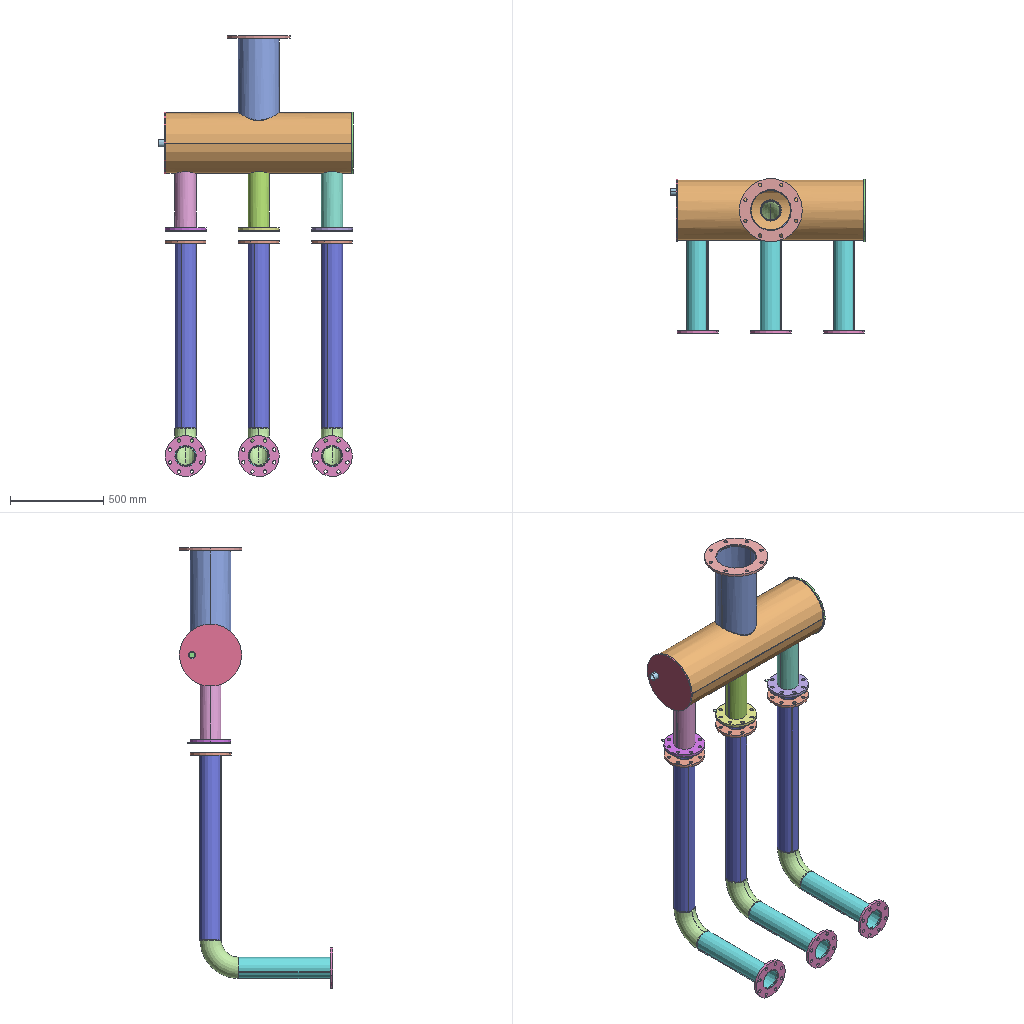Assembly | SolidWorks | 7 different items | 16 placed | box 1046 x 824 x 2365 mm
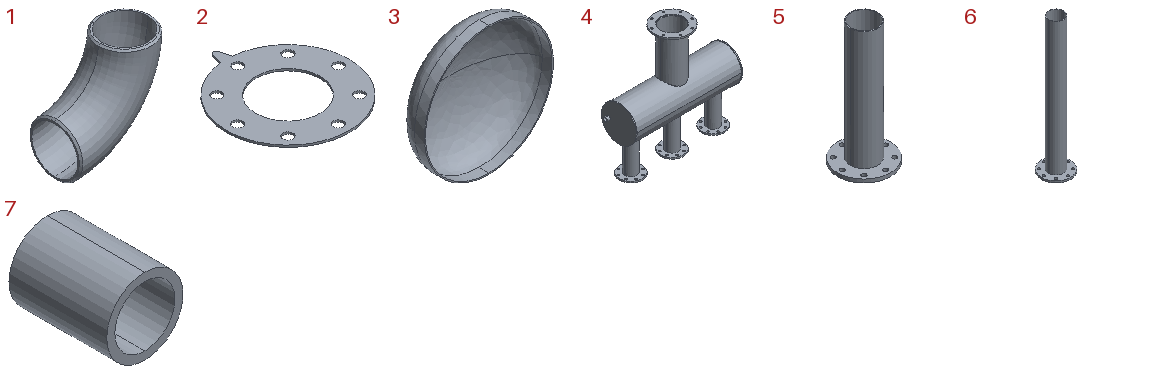Parts list (item | quantity | size | volume | features):
1 | x3 | 209.12 x 114.3 x 209.115 mm | 569487 mm3 | features Chamfer 1, Revolution 1
2 | x3 | 220 x 243.233 x 3.5 mm | 90689 mm3 | features Extrusion 1
3 | x2 | 325 x 106 x 325 mm | 399345 mm3 | features Revolution 2
4 | x1 | 1046 x 340 x 1046 mm | 7874309 mm3 | features ICE 8, 3DProfileFeature 4, Extrusion 1, MoveCopyBody 1, Stock 1, Sweep 1, WeldmentFeature 1
5 | x3 | 220 x 220 x 504 mm | 882758 mm3 | features Extrusion 1, ICE 1
6 | x3 | 220 x 220 x 1004 mm | 1407247 mm3 | features Extrusion 1, ICE 1
7 | x1 | 39 x 50 x 39 mm | 22597 mm3 | features 3DProfileFeature 1, Extrusion 1, HoleWzd 1
Mates (type | each side: item.copy, entity, surface, feature):
Concentric | 4.1 edge | 2.1 edge
Coincident | 4.1 face plane Boss-Extrude5 | 2.1 face plane Boss-Extrude1
Concentric | 4.1 face cylinder Boss-Extrude5 | 2.1 face cylinder Boss-Extrude1
Concentric | 2.1 edge | 6.1 edge
DistanceDim | 2.1 face plane Boss-Extrude1 | 6.1 face plane Boss-Extrude1
Concentric | 2.1 face cylinder Boss-Extrude1 | 6.1 face cylinder Boss-Extrude1
Concentric | 2.2 edge | 6.2 edge
DistanceDim | 2.2 face plane Boss-Extrude1 | 6.2 face plane Boss-Extrude1
Concentric | 2.2 face cylinder Boss-Extrude1 | 6.2 face cylinder Boss-Extrude1
DistanceDim | 2.3 face plane Boss-Extrude1 | 6.3 face plane Boss-Extrude1
Concentric | 2.3 face cylinder Boss-Extrude1 | 6.3 face cylinder Boss-Extrude1 | 2 times
Concentric | 6.1 edge | 1.1 edge
Coincident | 6.1 face plane Boss-Extrude2 | 1.1 face plane Revolve1
Parallel | 1.1 plane | assembly plane
Concentric | 6.2 edge | 1.2 edge
Coincident | 6.2 face plane Boss-Extrude2 | 1.2 face plane Revolve1
Parallel | 1.2 plane | assembly plane
Concentric | 6.3 edge | 1.3 edge
Coincident | 6.3 face plane Boss-Extrude2 | 1.3 face plane Revolve1
Parallel | 1.3 plane | assembly plane
Concentric | 1.1 edge | 5.1 edge
Coincident | 1.1 face plane Revolve1 | 5.1 face plane Boss-Extrude2
Concentric | 1.2 edge | 5.2 edge
Coincident | 1.2 face plane Revolve1 | 5.2 face plane Boss-Extrude2
Concentric | 1.3 edge | 5.3 edge
Coincident | 1.3 face plane Revolve1 | 5.3 face plane Boss-Extrude2
Concentric | 4.1 face cylinder Sweep-thin1 | 3.1 face cylinder Revolve2
Coincident | 4.1 face plane Sweep-thin1 | 3.1 face plane Revolve2
Concentric | 4.1 face cylinder Sweep-thin1 | 3.2 face cylinder Revolve2
Coincident | 4.1 face plane Sweep-thin1 | 3.2 face plane Revolve2
Parallel | 5.1 select_type:24 | assembly plane
Coincident | 4.1 face plane Boss-Extrude5 | 2.2 face plane Boss-Extrude1
Concentric | 4.1 face cylinder Boss-Extrude4 | 6.2 face cylinder Boss-Extrude2
Concentric | 4.1 face cylinder Boss-Extrude5 | 6.2 face cylinder Boss-Extrude1
Concentric | 4.1 face cylinder Boss-Extrude5 | 6.3 face cylinder Boss-Extrude1
Concentric | 4.1 face cylinder Boss-Extrude4 | 6.3 face cylinder Boss-Extrude2
Coincident | 4.1 face plane Boss-Extrude5 | 2.3 face plane Boss-Extrude1
Parallel | 5.2 select_type:24 | assembly plane
Parallel | 5.3 select_type:24 | assembly plane